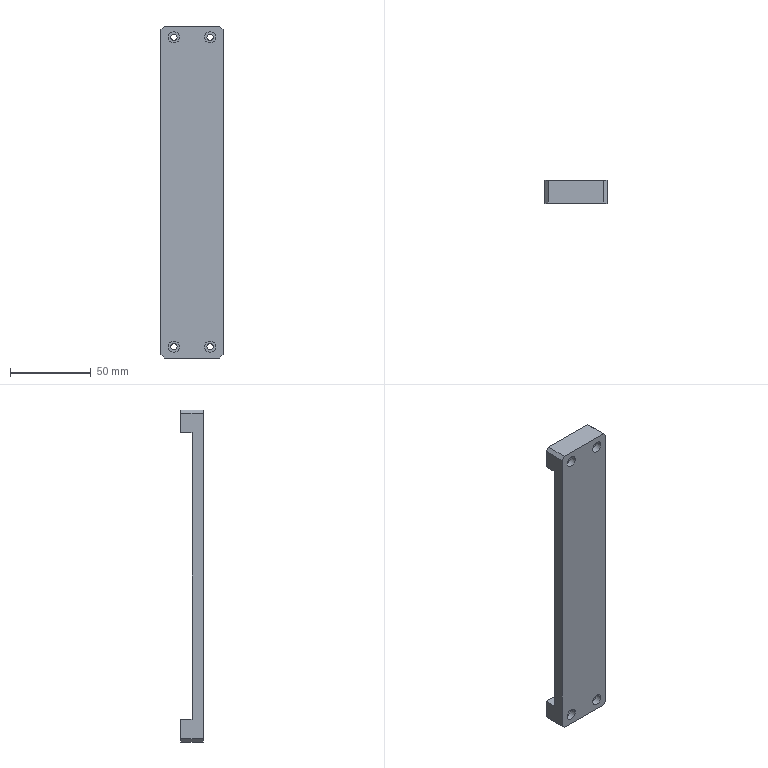Part | SolidWorks | features SplitBody 1 | 1 solid | 34 faces | box 38.5 x 14 x 205.8 mm | volume 61805 mm3 | plane 18 | cylinder 16 | commonest cylinder face diameters 3.85 x8 7 x8
STEP:
#1=CARTESIAN_POINT('',(1.625,218.849,-456.116));
#2=VERTEX_POINT('',#1);
#3=CARTESIAN_POINT('',(8.625,218.849,-456.116));
#4=VERTEX_POINT('',#3);
#5=CARTESIAN_POINT('',(5.125,218.849,-456.116));
#6=DIRECTION('',(0.,-1.,0.));
#7=DIRECTION('',(1.,0.,0.));
#8=AXIS2_PLACEMENT_3D('',#5,#6,#7);
#9=CIRCLE('',#8,3.5);
#10=EDGE_CURVE('',#2,#4,#9,.T.);
#11=ORIENTED_EDGE('',*,*,#10,.F.);
#12=CARTESIAN_POINT('',(1.625,214.859,-456.116));
#13=VERTEX_POINT('',#12);
#14=CARTESIAN_POINT('',(1.625,214.859,-456.116));
#15=DIRECTION('',(0.,-1.,0.));
#16=VECTOR('',#15,1000.);
#17=LINE('',#14,#16);
#18=EDGE_CURVE('',#2,#13,#17,.T.);
#19=ORIENTED_EDGE('',*,*,#18,.T.);
#20=CARTESIAN_POINT('',(8.625,214.859,-456.116));
#21=VERTEX_POINT('',#20);
#22=CARTESIAN_POINT('',(5.125,214.859,-456.116));
#23=DIRECTION('',(0.,-1.,0.));
#24=DIRECTION('',(1.,0.,0.));
#25=AXIS2_PLACEMENT_3D('',#22,#23,#24);
#26=CIRCLE('',#25,3.5);
#27=EDGE_CURVE('',#13,#21,#26,.T.);
#28=ORIENTED_EDGE('',*,*,#27,.T.);
#29=CARTESIAN_POINT('',(8.625,214.859,-456.116));
#30=DIRECTION('',(0.,-1.,0.));
#31=VECTOR('',#30,1000.);
#32=LINE('',#29,#31);
#33=EDGE_CURVE('',#4,#21,#32,.T.);
#34=ORIENTED_EDGE('',*,*,#33,.F.);
#35=EDGE_LOOP('',(#11,#19,#28,#34));
#36=FACE_OUTER_BOUND('',#35,.T.);
#37=CARTESIAN_POINT('',(5.125,214.859,-456.116));
#38=DIRECTION('',(0.,-1.,0.));
#39=DIRECTION('',(1.,0.,0.));
#40=AXIS2_PLACEMENT_3D('',#37,#38,#39);
#41=CYLINDRICAL_SURFACE('',#40,3.5);
#42=ADVANCED_FACE('',(#36),#41,.F.);
#43=CARTESIAN_POINT('',(3.2,228.859,-456.116));
#44=VERTEX_POINT('',#43);
#45=CARTESIAN_POINT('',(7.05,228.859,-456.116));
#46=VERTEX_POINT('',#45);
#47=CARTESIAN_POINT('',(5.125,228.859,-456.116));
#48=DIRECTION('',(0.,-1.,0.));
#49=DIRECTION('',(1.,0.,0.));
#50=AXIS2_PLACEMENT_3D('',#47,#48,#49);
#51=CIRCLE('',#50,1.925);
#52=EDGE_CURVE('',#44,#46,#51,.T.);
#53=ORIENTED_EDGE('',*,*,#52,.F.);
#54=CARTESIAN_POINT('',(3.2,218.849,-456.116));
#55=VERTEX_POINT('',#54);
#56=CARTESIAN_POINT('',(3.2,214.859,-456.116));
#57=DIRECTION('',(0.,-1.,0.));
#58=VECTOR('',#57,1000.);
#59=LINE('',#56,#58);
#60=EDGE_CURVE('',#44,#55,#59,.T.);
#61=ORIENTED_EDGE('',*,*,#60,.T.);
#62=CARTESIAN_POINT('',(7.05,218.849,-456.116));
#63=VERTEX_POINT('',#62);
#64=CARTESIAN_POINT('',(5.125,218.849,-456.116));
#65=DIRECTION('',(0.,-1.,0.));
#66=DIRECTION('',(1.,0.,0.));
#67=AXIS2_PLACEMENT_3D('',#64,#65,#66);
#68=CIRCLE('',#67,1.925);
#69=EDGE_CURVE('',#55,#63,#68,.T.);
#70=ORIENTED_EDGE('',*,*,#69,.T.);
#71=CARTESIAN_POINT('',(7.05,214.859,-456.116));
#72=DIRECTION('',(0.,-1.,0.));
#73=VECTOR('',#72,1000.);
#74=LINE('',#71,#73);
#75=EDGE_CURVE('',#46,#63,#74,.T.);
#76=ORIENTED_EDGE('',*,*,#75,.F.);
#77=EDGE_LOOP('',(#53,#61,#70,#76));
#78=FACE_OUTER_BOUND('',#77,.T.);
#79=CARTESIAN_POINT('',(5.125,214.859,-456.116));
#80=DIRECTION('',(0.,-1.,0.));
#81=DIRECTION('',(1.,0.,0.));
#82=AXIS2_PLACEMENT_3D('',#79,#80,#81);
#83=CYLINDRICAL_SURFACE('',#82,1.925);
#84=ADVANCED_FACE('',(#78),#83,.F.);
#85=CARTESIAN_POINT('',(24.025,218.849,-456.116));
#86=VERTEX_POINT('',#85);
#87=CARTESIAN_POINT('',(31.025,218.849,-456.116));
#88=VERTEX_POINT('',#87);
#89=CARTESIAN_POINT('',(27.525,218.849,-456.116));
#90=DIRECTION('',(0.,-1.,0.));
#91=DIRECTION('',(1.,0.,0.));
#92=AXIS2_PLACEMENT_3D('',#89,#90,#91);
#93=CIRCLE('',#92,3.5);
#94=EDGE_CURVE('',#86,#88,#93,.T.);
#95=ORIENTED_EDGE('',*,*,#94,.F.);
#96=CARTESIAN_POINT('',(24.025,214.859,-456.116));
#97=VERTEX_POINT('',#96);
#98=CARTESIAN_POINT('',(24.025,214.859,-456.116));
#99=DIRECTION('',(0.,-1.,0.));
#100=VECTOR('',#99,1000.);
#101=LINE('',#98,#100);
#102=EDGE_CURVE('',#86,#97,#101,.T.);
#103=ORIENTED_EDGE('',*,*,#102,.T.);
#104=CARTESIAN_POINT('',(31.025,214.859,-456.116));
#105=VERTEX_POINT('',#104);
#106=CARTESIAN_POINT('',(27.525,214.859,-456.116));
#107=DIRECTION('',(0.,-1.,0.));
#108=DIRECTION('',(1.,0.,0.));
#109=AXIS2_PLACEMENT_3D('',#106,#107,#108);
#110=CIRCLE('',#109,3.5);
#111=EDGE_CURVE('',#97,#105,#110,.T.);
#112=ORIENTED_EDGE('',*,*,#111,.T.);
#113=CARTESIAN_POINT('',(31.025,214.859,-456.116));
#114=DIRECTION('',(0.,-1.,0.));
#115=VECTOR('',#114,1000.);
#116=LINE('',#113,#115);
#117=EDGE_CURVE('',#88,#105,#116,.T.);
#118=ORIENTED_EDGE('',*,*,#117,.F.);
#119=EDGE_LOOP('',(#95,#103,#112,#118));
#120=FACE_OUTER_BOUND('',#119,.T.);
#121=CARTESIAN_POINT('',(27.525,214.859,-456.116));
#122=DIRECTION('',(0.,-1.,0.));
#123=DIRECTION('',(1.,0.,0.));
#124=AXIS2_PLACEMENT_3D('',#121,#122,#123);
#125=CYLINDRICAL_SURFACE('',#124,3.5);
#126=ADVANCED_FACE('',(#120),#125,.F.);
#127=CARTESIAN_POINT('',(25.6,228.859,-456.116));
#128=VERTEX_POINT('',#127);
#129=CARTESIAN_POINT('',(29.45,228.859,-456.116));
#130=VERTEX_POINT('',#129);
#131=CARTESIAN_POINT('',(27.525,228.859,-456.116));
#132=DIRECTION('',(0.,-1.,0.));
#133=DIRECTION('',(1.,0.,0.));
#134=AXIS2_PLACEMENT_3D('',#131,#132,#133);
#135=CIRCLE('',#134,1.925);
#136=EDGE_CURVE('',#128,#130,#135,.T.);
#137=ORIENTED_EDGE('',*,*,#136,.F.);
#138=CARTESIAN_POINT('',(25.6,218.849,-456.116));
#139=VERTEX_POINT('',#138);
#140=CARTESIAN_POINT('',(25.6,214.859,-456.116));
#141=DIRECTION('',(0.,-1.,0.));
#142=VECTOR('',#141,1000.);
#143=LINE('',#140,#142);
#144=EDGE_CURVE('',#128,#139,#143,.T.);
#145=ORIENTED_EDGE('',*,*,#144,.T.);
#146=CARTESIAN_POINT('',(29.45,218.849,-456.116));
#147=VERTEX_POINT('',#146);
#148=CARTESIAN_POINT('',(27.525,218.849,-456.116));
#149=DIRECTION('',(0.,-1.,0.));
#150=DIRECTION('',(1.,0.,0.));
#151=AXIS2_PLACEMENT_3D('',#148,#149,#150);
#152=CIRCLE('',#151,1.925);
#153=EDGE_CURVE('',#139,#147,#152,.T.);
#154=ORIENTED_EDGE('',*,*,#153,.T.);
#155=CARTESIAN_POINT('',(29.45,214.859,-456.116));
#156=DIRECTION('',(0.,-1.,0.));
#157=VECTOR('',#156,1000.);
#158=LINE('',#155,#157);
#159=EDGE_CURVE('',#130,#147,#158,.T.);
#160=ORIENTED_EDGE('',*,*,#159,.F.);
#161=EDGE_LOOP('',(#137,#145,#154,#160));
#162=FACE_OUTER_BOUND('',#161,.T.);
#163=CARTESIAN_POINT('',(27.525,214.859,-456.116));
#164=DIRECTION('',(0.,-1.,0.));
#165=DIRECTION('',(1.,0.,0.));
#166=AXIS2_PLACEMENT_3D('',#163,#164,#165);
#167=CYLINDRICAL_SURFACE('',#166,1.925);
#168=ADVANCED_FACE('',(#162),#167,.F.);
#169=CARTESIAN_POINT('',(1.625,218.849,-264.316));
#170=VERTEX_POINT('',#169);
#171=CARTESIAN_POINT('',(8.625,218.849,-264.316));
#172=VERTEX_POINT('',#171);
#173=CARTESIAN_POINT('',(5.125,218.849,-264.316));
#174=DIRECTION('',(0.,-1.,0.));
#175=DIRECTION('',(1.,0.,0.));
#176=AXIS2_PLACEMENT_3D('',#173,#174,#175);
#177=CIRCLE('',#176,3.5);
#178=EDGE_CURVE('',#170,#172,#177,.T.);
#179=ORIENTED_EDGE('',*,*,#178,.F.);
#180=CARTESIAN_POINT('',(1.625,214.859,-264.316));
#181=VERTEX_POINT('',#180);
#182=CARTESIAN_POINT('',(1.625,214.859,-264.316));
#183=DIRECTION('',(0.,-1.,0.));
#184=VECTOR('',#183,1000.);
#185=LINE('',#182,#184);
#186=EDGE_CURVE('',#170,#181,#185,.T.);
#187=ORIENTED_EDGE('',*,*,#186,.T.);
#188=CARTESIAN_POINT('',(8.625,214.859,-264.316));
#189=VERTEX_POINT('',#188);
#190=CARTESIAN_POINT('',(5.125,214.859,-264.316));
#191=DIRECTION('',(0.,-1.,0.));
#192=DIRECTION('',(1.,0.,0.));
#193=AXIS2_PLACEMENT_3D('',#190,#191,#192);
#194=CIRCLE('',#193,3.5);
#195=EDGE_CURVE('',#181,#189,#194,.T.);
#196=ORIENTED_EDGE('',*,*,#195,.T.);
#197=CARTESIAN_POINT('',(8.625,214.859,-264.316));
#198=DIRECTION('',(0.,-1.,0.));
#199=VECTOR('',#198,1000.);
#200=LINE('',#197,#199);
#201=EDGE_CURVE('',#172,#189,#200,.T.);
#202=ORIENTED_EDGE('',*,*,#201,.F.);
#203=EDGE_LOOP('',(#179,#187,#196,#202));
#204=FACE_OUTER_BOUND('',#203,.T.);
#205=CARTESIAN_POINT('',(5.125,214.859,-264.316));
#206=DIRECTION('',(0.,-1.,0.));
#207=DIRECTION('',(1.,0.,0.));
#208=AXIS2_PLACEMENT_3D('',#205,#206,#207);
#209=CYLINDRICAL_SURFACE('',#208,3.5);
#210=ADVANCED_FACE('',(#204),#209,.F.);
#211=CARTESIAN_POINT('',(3.2,228.859,-264.316));
#212=VERTEX_POINT('',#211);
#213=CARTESIAN_POINT('',(7.05,228.859,-264.316));
#214=VERTEX_POINT('',#213);
#215=CARTESIAN_POINT('',(5.125,228.859,-264.316));
#216=DIRECTION('',(0.,-1.,0.));
#217=DIRECTION('',(1.,0.,0.));
#218=AXIS2_PLACEMENT_3D('',#215,#216,#217);
#219=CIRCLE('',#218,1.925);
#220=EDGE_CURVE('',#212,#214,#219,.T.);
#221=ORIENTED_EDGE('',*,*,#220,.F.);
#222=CARTESIAN_POINT('',(3.2,218.849,-264.316));
#223=VERTEX_POINT('',#222);
#224=CARTESIAN_POINT('',(3.2,214.859,-264.316));
#225=DIRECTION('',(0.,-1.,0.));
#226=VECTOR('',#225,1000.);
#227=LINE('',#224,#226);
#228=EDGE_CURVE('',#212,#223,#227,.T.);
#229=ORIENTED_EDGE('',*,*,#228,.T.);
#230=CARTESIAN_POINT('',(7.05,218.849,-264.316));
#231=VERTEX_POINT('',#230);
#232=CARTESIAN_POINT('',(5.125,218.849,-264.316));
#233=DIRECTION('',(0.,-1.,0.));
#234=DIRECTION('',(1.,0.,0.));
#235=AXIS2_PLACEMENT_3D('',#232,#233,#234);
#236=CIRCLE('',#235,1.925);
#237=EDGE_CURVE('',#223,#231,#236,.T.);
#238=ORIENTED_EDGE('',*,*,#237,.T.);
#239=CARTESIAN_POINT('',(7.05,214.859,-264.316));
#240=DIRECTION('',(0.,-1.,0.));
#241=VECTOR('',#240,1000.);
#242=LINE('',#239,#241);
#243=EDGE_CURVE('',#214,#231,#242,.T.);
#244=ORIENTED_EDGE('',*,*,#243,.F.);
#245=EDGE_LOOP('',(#221,#229,#238,#244));
#246=FACE_OUTER_BOUND('',#245,.T.);
#247=CARTESIAN_POINT('',(5.125,214.859,-264.316));
#248=DIRECTION('',(0.,-1.,0.));
#249=DIRECTION('',(1.,0.,0.));
#250=AXIS2_PLACEMENT_3D('',#247,#248,#249);
#251=CYLINDRICAL_SURFACE('',#250,1.925);
#252=ADVANCED_FACE('',(#246),#251,.F.);
#253=CARTESIAN_POINT('',(24.025,218.849,-264.316));
#254=VERTEX_POINT('',#253);
#255=CARTESIAN_POINT('',(31.025,218.849,-264.316));
#256=VERTEX_POINT('',#255);
#257=CARTESIAN_POINT('',(27.525,218.849,-264.316));
#258=DIRECTION('',(0.,-1.,0.));
#259=DIRECTION('',(1.,0.,0.));
#260=AXIS2_PLACEMENT_3D('',#257,#258,#259);
#261=CIRCLE('',#260,3.5);
#262=EDGE_CURVE('',#254,#256,#261,.T.);
#263=ORIENTED_EDGE('',*,*,#262,.F.);
#264=CARTESIAN_POINT('',(24.025,214.859,-264.316));
#265=VERTEX_POINT('',#264);
#266=CARTESIAN_POINT('',(24.025,214.859,-264.316));
#267=DIRECTION('',(0.,-1.,0.));
#268=VECTOR('',#267,1000.);
#269=LINE('',#266,#268);
#270=EDGE_CURVE('',#254,#265,#269,.T.);
#271=ORIENTED_EDGE('',*,*,#270,.T.);
#272=CARTESIAN_POINT('',(31.025,214.859,-264.316));
#273=VERTEX_POINT('',#272);
#274=CARTESIAN_POINT('',(27.525,214.859,-264.316));
#275=DIRECTION('',(0.,-1.,0.));
#276=DIRECTION('',(1.,0.,0.));
#277=AXIS2_PLACEMENT_3D('',#274,#275,#276);
#278=CIRCLE('',#277,3.5);
#279=EDGE_CURVE('',#265,#273,#278,.T.);
#280=ORIENTED_EDGE('',*,*,#279,.T.);
#281=CARTESIAN_POINT('',(31.025,214.859,-264.316));
#282=DIRECTION('',(0.,-1.,0.));
#283=VECTOR('',#282,1000.);
#284=LINE('',#281,#283);
#285=EDGE_CURVE('',#256,#273,#284,.T.);
#286=ORIENTED_EDGE('',*,*,#285,.F.);
#287=EDGE_LOOP('',(#263,#271,#280,#286));
#288=FACE_OUTER_BOUND('',#287,.T.);
#289=CARTESIAN_POINT('',(27.525,214.859,-264.316));
#290=DIRECTION('',(0.,-1.,0.));
#291=DIRECTION('',(1.,0.,0.));
#292=AXIS2_PLACEMENT_3D('',#289,#290,#291);
#293=CYLINDRICAL_SURFACE('',#292,3.5);
#294=ADVANCED_FACE('',(#288),#293,.F.);
#295=CARTESIAN_POINT('',(25.6,228.859,-264.316));
#296=VERTEX_POINT('',#295);
#297=CARTESIAN_POINT('',(29.45,228.859,-264.316));
#298=VERTEX_POINT('',#297);
#299=CARTESIAN_POINT('',(27.525,228.859,-264.316));
#300=DIRECTION('',(0.,-1.,0.));
#301=DIRECTION('',(1.,0.,0.));
#302=AXIS2_PLACEMENT_3D('',#299,#300,#301);
#303=CIRCLE('',#302,1.925);
#304=EDGE_CURVE('',#296,#298,#303,.T.);
#305=ORIENTED_EDGE('',*,*,#304,.F.);
#306=CARTESIAN_POINT('',(25.6,218.849,-264.316));
#307=VERTEX_POINT('',#306);
#308=CARTESIAN_POINT('',(25.6,214.859,-264.316));
#309=DIRECTION('',(0.,-1.,0.));
#310=VECTOR('',#309,1000.);
#311=LINE('',#308,#310);
#312=EDGE_CURVE('',#296,#307,#311,.T.);
#313=ORIENTED_EDGE('',*,*,#312,.T.);
#314=CARTESIAN_POINT('',(29.45,218.849,-264.316));
#315=VERTEX_POINT('',#314);
#316=CARTESIAN_POINT('',(27.525,218.849,-264.316));
#317=DIRECTION('',(0.,-1.,0.));
#318=DIRECTION('',(1.,0.,0.));
#319=AXIS2_PLACEMENT_3D('',#316,#317,#318);
#320=CIRCLE('',#319,1.925);
#321=EDGE_CURVE('',#307,#315,#320,.T.);
#322=ORIENTED_EDGE('',*,*,#321,.T.);
#323=CARTESIAN_POINT('',(29.45,214.859,-264.316));
#324=DIRECTION('',(0.,-1.,0.));
#325=VECTOR('',#324,1000.);
#326=LINE('',#323,#325);
#327=EDGE_CURVE('',#298,#315,#326,.T.);
#328=ORIENTED_EDGE('',*,*,#327,.F.);
#329=EDGE_LOOP('',(#305,#313,#322,#328));
#330=FACE_OUTER_BOUND('',#329,.T.);
#331=CARTESIAN_POINT('',(27.525,214.859,-264.316));
#332=DIRECTION('',(0.,-1.,0.));
#333=DIRECTION('',(1.,0.,0.));
#334=AXIS2_PLACEMENT_3D('',#331,#332,#333);
#335=CYLINDRICAL_SURFACE('',#334,1.925);
#336=ADVANCED_FACE('',(#330),#335,.F.);
#337=CARTESIAN_POINT('',(-0.8247,228.859,-463.116));
#338=VERTEX_POINT('',#337);
#339=CARTESIAN_POINT('',(33.475,228.859,-463.116));
#340=VERTEX_POINT('',#339);
#341=CARTESIAN_POINT('',(-2.925,228.859,-463.116));
#342=DIRECTION('',(1.,0.,0.));
#343=VECTOR('',#342,1000.);
#344=LINE('',#341,#343);
#345=EDGE_CURVE('',#338,#340,#344,.T.);
#346=ORIENTED_EDGE('',*,*,#345,.T.);
#347=CARTESIAN_POINT('',(33.475,214.859,-463.116));
#348=VERTEX_POINT('',#347);
#349=CARTESIAN_POINT('',(33.475,214.859,-463.116));
#350=DIRECTION('',(0.,-1.,0.));
#351=VECTOR('',#350,1000.);
#352=LINE('',#349,#351);
#353=EDGE_CURVE('',#340,#348,#352,.T.);
#354=ORIENTED_EDGE('',*,*,#353,.T.);
#355=CARTESIAN_POINT('',(-0.8247,214.859,-463.116));
#356=VERTEX_POINT('',#355);
#357=CARTESIAN_POINT('',(-2.925,214.859,-463.116));
#358=DIRECTION('',(1.,0.,0.));
#359=VECTOR('',#358,1000.);
#360=LINE('',#357,#359);
#361=EDGE_CURVE('',#356,#348,#360,.T.);
#362=ORIENTED_EDGE('',*,*,#361,.F.);
#363=CARTESIAN_POINT('',(-0.8247,214.859,-463.116));
#364=DIRECTION('',(0.,1.,0.));
#365=VECTOR('',#364,1000.);
#366=LINE('',#363,#365);
#367=EDGE_CURVE('',#356,#338,#366,.T.);
#368=ORIENTED_EDGE('',*,*,#367,.T.);
#369=EDGE_LOOP('',(#346,#354,#362,#368));
#370=FACE_OUTER_BOUND('',#369,.T.);
#371=CARTESIAN_POINT('',(-2.925,214.859,-463.116));
#372=DIRECTION('',(0.,0.,1.));
#373=DIRECTION('',(1.,0.,0.));
#374=AXIS2_PLACEMENT_3D('',#371,#372,#373);
#375=PLANE('',#374);
#376=ADVANCED_FACE('',(#370),#375,.F.);
#377=CARTESIAN_POINT('',(5.125,214.859,-456.116));
#378=DIRECTION('',(0.,-1.,0.));
#379=DIRECTION('',(1.,0.,0.));
#380=AXIS2_PLACEMENT_3D('',#377,#378,#379);
#381=CIRCLE('',#380,3.5);
#382=EDGE_CURVE('',#21,#13,#381,.T.);
#383=ORIENTED_EDGE('',*,*,#382,.F.);
#384=ORIENTED_EDGE('',*,*,#27,.F.);
#385=EDGE_LOOP('',(#383,#384));
#386=FACE_BOUND('',#385,.T.);
#387=CARTESIAN_POINT('',(27.525,214.859,-456.116));
#388=DIRECTION('',(0.,-1.,0.));
#389=DIRECTION('',(1.,0.,0.));
#390=AXIS2_PLACEMENT_3D('',#387,#388,#389);
#391=CIRCLE('',#390,3.5);
#392=EDGE_CURVE('',#105,#97,#391,.T.);
#393=ORIENTED_EDGE('',*,*,#392,.F.);
#394=ORIENTED_EDGE('',*,*,#111,.F.);
#395=EDGE_LOOP('',(#393,#394));
#396=FACE_BOUND('',#395,.T.);
#397=CARTESIAN_POINT('',(5.125,214.859,-264.316));
#398=DIRECTION('',(0.,-1.,0.));
#399=DIRECTION('',(1.,0.,0.));
#400=AXIS2_PLACEMENT_3D('',#397,#398,#399);
#401=CIRCLE('',#400,3.5);
#402=EDGE_CURVE('',#189,#181,#401,.T.);
#403=ORIENTED_EDGE('',*,*,#402,.F.);
#404=ORIENTED_EDGE('',*,*,#195,.F.);
#405=EDGE_LOOP('',(#403,#404));
#406=FACE_BOUND('',#405,.T.);
#407=CARTESIAN_POINT('',(27.525,214.859,-264.316));
#408=DIRECTION('',(0.,-1.,0.));
#409=DIRECTION('',(1.,0.,0.));
#410=AXIS2_PLACEMENT_3D('',#407,#408,#409);
#411=CIRCLE('',#410,3.5);
#412=EDGE_CURVE('',#273,#265,#411,.T.);
#413=ORIENTED_EDGE('',*,*,#412,.F.);
#414=ORIENTED_EDGE('',*,*,#279,.F.);
#415=EDGE_LOOP('',(#413,#414));
#416=FACE_BOUND('',#415,.T.);
#417=CARTESIAN_POINT('',(35.575,214.859,-461.016));
#418=VERTEX_POINT('',#417);
#419=CARTESIAN_POINT('',(35.575,214.859,-259.416));
#420=VERTEX_POINT('',#419);
#421=CARTESIAN_POINT('',(35.575,214.859,-463.116));
#422=DIRECTION('',(0.,0.,1.));
#423=VECTOR('',#422,1000.);
#424=LINE('',#421,#423);
#425=EDGE_CURVE('',#418,#420,#424,.T.);
#426=ORIENTED_EDGE('',*,*,#425,.T.);
#427=CARTESIAN_POINT('',(33.475,214.859,-257.316));
#428=VERTEX_POINT('',#427);
#429=CARTESIAN_POINT('',(33.475,214.859,-257.316));
#430=DIRECTION('',(-0.7071,0.,0.7071));
#431=VECTOR('',#430,1000.);
#432=LINE('',#429,#431);
#433=EDGE_CURVE('',#420,#428,#432,.T.);
#434=ORIENTED_EDGE('',*,*,#433,.T.);
#435=CARTESIAN_POINT('',(-0.8247,214.859,-257.316));
#436=VERTEX_POINT('',#435);
#437=CARTESIAN_POINT('',(-2.925,214.859,-257.316));
#438=DIRECTION('',(1.,0.,0.));
#439=VECTOR('',#438,1000.);
#440=LINE('',#437,#439);
#441=EDGE_CURVE('',#436,#428,#440,.T.);
#442=ORIENTED_EDGE('',*,*,#441,.F.);
#443=CARTESIAN_POINT('',(-2.925,214.859,-259.416));
#444=VERTEX_POINT('',#443);
#445=CARTESIAN_POINT('',(-2.925,214.859,-259.416));
#446=DIRECTION('',(-0.7071,0.,-0.7071));
#447=VECTOR('',#446,1000.);
#448=LINE('',#445,#447);
#449=EDGE_CURVE('',#436,#444,#448,.T.);
#450=ORIENTED_EDGE('',*,*,#449,.T.);
#451=CARTESIAN_POINT('',(-2.925,214.859,-461.016));
#452=VERTEX_POINT('',#451);
#453=CARTESIAN_POINT('',(-2.925,214.859,-463.116));
#454=DIRECTION('',(0.,0.,1.));
#455=VECTOR('',#454,1000.);
#456=LINE('',#453,#455);
#457=EDGE_CURVE('',#452,#444,#456,.T.);
#458=ORIENTED_EDGE('',*,*,#457,.F.);
#459=CARTESIAN_POINT('',(-2.925,214.859,-461.016));
#460=DIRECTION('',(0.7071,0.,-0.7071));
#461=VECTOR('',#460,1000.);
#462=LINE('',#459,#461);
#463=EDGE_CURVE('',#452,#356,#462,.T.);
#464=ORIENTED_EDGE('',*,*,#463,.T.);
#465=ORIENTED_EDGE('',*,*,#361,.T.);
#466=CARTESIAN_POINT('',(33.475,214.859,-463.116));
#467=DIRECTION('',(0.7071,0.,0.7071));
#468=VECTOR('',#467,1000.);
#469=LINE('',#466,#468);
#470=EDGE_CURVE('',#348,#418,#469,.T.);
#471=ORIENTED_EDGE('',*,*,#470,.T.);
#472=EDGE_LOOP('',(#426,#434,#442,#450,#458,#464,#465,#471));
#473=FACE_OUTER_BOUND('',#472,.T.);
#474=CARTESIAN_POINT('',(-2.925,214.859,-463.116));
#475=DIRECTION('',(0.,1.,0.));
#476=DIRECTION('',(-1.,0.,0.));
#477=AXIS2_PLACEMENT_3D('',#474,#475,#476);
#478=PLANE('',#477);
#479=ADVANCED_FACE('',(#386,#396,#406,#416,#473),#478,.F.);
#480=ORIENTED_EDGE('',*,*,#441,.T.);
#481=CARTESIAN_POINT('',(33.475,228.859,-257.316));
#482=VERTEX_POINT('',#481);
#483=CARTESIAN_POINT('',(33.475,228.859,-257.316));
#484=DIRECTION('',(0.,1.,0.));
#485=VECTOR('',#484,1000.);
#486=LINE('',#483,#485);
#487=EDGE_CURVE('',#428,#482,#486,.T.);
#488=ORIENTED_EDGE('',*,*,#487,.T.);
#489=CARTESIAN_POINT('',(-0.8247,228.859,-257.316));
#490=VERTEX_POINT('',#489);
#491=CARTESIAN_POINT('',(-2.925,228.859,-257.316));
#492=DIRECTION('',(1.,0.,0.));
#493=VECTOR('',#492,1000.);
#494=LINE('',#491,#493);
#495=EDGE_CURVE('',#490,#482,#494,.T.);
#496=ORIENTED_EDGE('',*,*,#495,.F.);
#497=CARTESIAN_POINT('',(-0.8247,214.859,-257.316));
#498=DIRECTION('',(0.,-1.,0.));
#499=VECTOR('',#498,1000.);
#500=LINE('',#497,#499);
#501=EDGE_CURVE('',#490,#436,#500,.T.);
#502=ORIENTED_EDGE('',*,*,#501,.T.);
#503=EDGE_LOOP('',(#480,#488,#496,#502));
#504=FACE_OUTER_BOUND('',#503,.T.);
#505=CARTESIAN_POINT('',(-2.925,214.859,-257.316));
#506=DIRECTION('',(0.,0.,-1.));
#507=DIRECTION('',(-1.,0.,0.));
#508=AXIS2_PLACEMENT_3D('',#505,#506,#507);
#509=PLANE('',#508);
#510=ADVANCED_FACE('',(#504),#509,.F.);
#511=CARTESIAN_POINT('',(5.125,228.859,-264.316));
#512=DIRECTION('',(0.,-1.,0.));
#513=DIRECTION('',(1.,0.,0.));
#514=AXIS2_PLACEMENT_3D('',#511,#512,#513);
#515=CIRCLE('',#514,1.925);
#516=EDGE_CURVE('',#214,#212,#515,.T.);
#517=ORIENTED_EDGE('',*,*,#516,.T.);
#518=ORIENTED_EDGE('',*,*,#220,.T.);
#519=EDGE_LOOP('',(#517,#518));
#520=FACE_BOUND('',#519,.T.);
#521=CARTESIAN_POINT('',(27.525,228.859,-264.316));
#522=DIRECTION('',(0.,-1.,0.));
#523=DIRECTION('',(1.,0.,0.));
#524=AXIS2_PLACEMENT_3D('',#521,#522,#523);
#525=CIRCLE('',#524,1.925);
#526=EDGE_CURVE('',#298,#296,#525,.T.);
#527=ORIENTED_EDGE('',*,*,#526,.T.);
#528=ORIENTED_EDGE('',*,*,#304,.T.);
#529=EDGE_LOOP('',(#527,#528));
#530=FACE_BOUND('',#529,.T.);
#531=ORIENTED_EDGE('',*,*,#495,.T.);
#532=CARTESIAN_POINT('',(35.575,228.859,-259.416));
#533=VERTEX_POINT('',#532);
#534=CARTESIAN_POINT('',(33.475,228.859,-257.316));
#535=DIRECTION('',(0.7071,0.,-0.7071));
#536=VECTOR('',#535,1000.);
#537=LINE('',#534,#536);
#538=EDGE_CURVE('',#482,#533,#537,.T.);
#539=ORIENTED_EDGE('',*,*,#538,.T.);
#540=CARTESIAN_POINT('',(35.575,228.859,-271.316));
#541=VERTEX_POINT('',#540);
#542=CARTESIAN_POINT('',(35.575,228.859,-271.316));
#543=DIRECTION('',(0.,0.,-1.));
#544=VECTOR('',#543,1000.);
#545=LINE('',#542,#544);
#546=EDGE_CURVE('',#533,#541,#545,.T.);
#547=ORIENTED_EDGE('',*,*,#546,.T.);
#548=CARTESIAN_POINT('',(-2.925,228.859,-271.316));
#549=VERTEX_POINT('',#548);
#550=CARTESIAN_POINT('',(-2.925,228.859,-271.316));
#551=DIRECTION('',(1.,0.,0.));
#552=VECTOR('',#551,1000.);
#553=LINE('',#550,#552);
#554=EDGE_CURVE('',#549,#541,#553,.T.);
#555=ORIENTED_EDGE('',*,*,#554,.F.);
#556=CARTESIAN_POINT('',(-2.925,228.859,-259.416));
#557=VERTEX_POINT('',#556);
#558=CARTESIAN_POINT('',(-2.925,228.859,-271.316));
#559=DIRECTION('',(0.,0.,-1.));
#560=VECTOR('',#559,1000.);
#561=LINE('',#558,#560);
#562=EDGE_CURVE('',#557,#549,#561,.T.);
#563=ORIENTED_EDGE('',*,*,#562,.F.);
#564=CARTESIAN_POINT('',(-2.925,228.859,-259.416));
#565=DIRECTION('',(0.7071,0.,0.7071));
#566=VECTOR('',#565,1000.);
#567=LINE('',#564,#566);
#568=EDGE_CURVE('',#557,#490,#567,.T.);
#569=ORIENTED_EDGE('',*,*,#568,.T.);
#570=EDGE_LOOP('',(#531,#539,#547,#555,#563,#569));
#571=FACE_OUTER_BOUND('',#570,.T.);
#572=CARTESIAN_POINT('',(-2.925,228.859,-271.316));
#573=DIRECTION('',(0.,-1.,0.));
#574=DIRECTION('',(1.,0.,0.));
#575=AXIS2_PLACEMENT_3D('',#572,#573,#574);
#576=PLANE('',#575);
#577=ADVANCED_FACE('',(#520,#530,#571),#576,.F.);
#578=CARTESIAN_POINT('',(35.575,221.859,-271.316));
#579=VERTEX_POINT('',#578);
#580=CARTESIAN_POINT('',(35.575,228.859,-271.316));
#581=DIRECTION('',(0.,-1.,0.));
#582=VECTOR('',#581,1000.);
#583=LINE('',#580,#582);
#584=EDGE_CURVE('',#541,#579,#583,.T.);
#585=ORIENTED_EDGE('',*,*,#584,.T.);
#586=CARTESIAN_POINT('',(-2.925,221.859,-271.316));
#587=VERTEX_POINT('',#586);
#588=CARTESIAN_POINT('',(-2.925,221.859,-271.316));
#589=DIRECTION('',(1.,0.,0.));
#590=VECTOR('',#589,1000.);
#591=LINE('',#588,#590);
#592=EDGE_CURVE('',#587,#579,#591,.T.);
#593=ORIENTED_EDGE('',*,*,#592,.F.);
#594=CARTESIAN_POINT('',(-2.925,228.859,-271.316));
#595=DIRECTION('',(0.,-1.,0.));
#596=VECTOR('',#595,1000.);
#597=LINE('',#594,#596);
#598=EDGE_CURVE('',#549,#587,#597,.T.);
#599=ORIENTED_EDGE('',*,*,#598,.F.);
#600=ORIENTED_EDGE('',*,*,#554,.T.);
#601=EDGE_LOOP('',(#585,#593,#599,#600));
#602=FACE_OUTER_BOUND('',#601,.T.);
#603=CARTESIAN_POINT('',(-2.925,228.859,-271.316));
#604=DIRECTION('',(0.,0.,1.));
#605=DIRECTION('',(1.,0.,0.));
#606=AXIS2_PLACEMENT_3D('',#603,#604,#605);
#607=PLANE('',#606);
#608=ADVANCED_FACE('',(#602),#607,.F.);
#609=CARTESIAN_POINT('',(35.575,221.859,-449.116));
#610=VERTEX_POINT('',#609);
#611=CARTESIAN_POINT('',(35.575,221.859,-449.116));
#612=DIRECTION('',(0.,0.,-1.));
#613=VECTOR('',#612,1000.);
#614=LINE('',#611,#613);
#615=EDGE_CURVE('',#579,#610,#614,.T.);
#616=ORIENTED_EDGE('',*,*,#615,.T.);
#617=CARTESIAN_POINT('',(-2.925,221.859,-449.116));
#618=VERTEX_POINT('',#617);
#619=CARTESIAN_POINT('',(-2.925,221.859,-449.116));
#620=DIRECTION('',(1.,0.,0.));
#621=VECTOR('',#620,1000.);
#622=LINE('',#619,#621);
#623=EDGE_CURVE('',#618,#610,#622,.T.);
#624=ORIENTED_EDGE('',*,*,#623,.F.);
#625=CARTESIAN_POINT('',(-2.925,221.859,-449.116));
#626=DIRECTION('',(0.,0.,-1.));
#627=VECTOR('',#626,1000.);
#628=LINE('',#625,#627);
#629=EDGE_CURVE('',#587,#618,#628,.T.);
#630=ORIENTED_EDGE('',*,*,#629,.F.);
#631=ORIENTED_EDGE('',*,*,#592,.T.);
#632=EDGE_LOOP('',(#616,#624,#630,#631));
#633=FACE_OUTER_BOUND('',#632,.T.);
#634=CARTESIAN_POINT('',(-2.925,221.859,-449.116));
#635=DIRECTION('',(0.,-1.,0.));
#636=DIRECTION('',(1.,0.,0.));
#637=AXIS2_PLACEMENT_3D('',#634,#635,#636);
#638=PLANE('',#637);
#639=ADVANCED_FACE('',(#633),#638,.F.);
#640=CARTESIAN_POINT('',(35.575,228.859,-449.116));
#641=VERTEX_POINT('',#640);
#642=CARTESIAN_POINT('',(35.575,228.859,-449.116));
#643=DIRECTION('',(0.,1.,0.));
#644=VECTOR('',#643,1000.);
#645=LINE('',#642,#644);
#646=EDGE_CURVE('',#610,#641,#645,.T.);
#647=ORIENTED_EDGE('',*,*,#646,.T.);
#648=CARTESIAN_POINT('',(-2.925,228.859,-449.116));
#649=VERTEX_POINT('',#648);
#650=CARTESIAN_POINT('',(-2.925,228.859,-449.116));
#651=DIRECTION('',(1.,0.,0.));
#652=VECTOR('',#651,1000.);
#653=LINE('',#650,#652);
#654=EDGE_CURVE('',#649,#641,#653,.T.);
#655=ORIENTED_EDGE('',*,*,#654,.F.);
#656=CARTESIAN_POINT('',(-2.925,228.859,-449.116));
#657=DIRECTION('',(0.,1.,0.));
#658=VECTOR('',#657,1000.);
#659=LINE('',#656,#658);
#660=EDGE_CURVE('',#618,#649,#659,.T.);
#661=ORIENTED_EDGE('',*,*,#660,.F.);
#662=ORIENTED_EDGE('',*,*,#623,.T.);
#663=EDGE_LOOP('',(#647,#655,#661,#662));
#664=FACE_OUTER_BOUND('',#663,.T.);
#665=CARTESIAN_POINT('',(-2.925,228.859,-449.116));
#666=DIRECTION('',(0.,0.,-1.));
#667=DIRECTION('',(-1.,0.,0.));
#668=AXIS2_PLACEMENT_3D('',#665,#666,#667);
#669=PLANE('',#668);
#670=ADVANCED_FACE('',(#664),#669,.F.);
#671=CARTESIAN_POINT('',(5.125,228.859,-456.116));
#672=DIRECTION('',(0.,-1.,0.));
#673=DIRECTION('',(1.,0.,0.));
#674=AXIS2_PLACEMENT_3D('',#671,#672,#673);
#675=CIRCLE('',#674,1.925);
#676=EDGE_CURVE('',#46,#44,#675,.T.);
#677=ORIENTED_EDGE('',*,*,#676,.T.);
#678=ORIENTED_EDGE('',*,*,#52,.T.);
#679=EDGE_LOOP('',(#677,#678));
#680=FACE_BOUND('',#679,.T.);
#681=CARTESIAN_POINT('',(27.525,228.859,-456.116));
#682=DIRECTION('',(0.,-1.,0.));
#683=DIRECTION('',(1.,0.,0.));
#684=AXIS2_PLACEMENT_3D('',#681,#682,#683);
#685=CIRCLE('',#684,1.925);
#686=EDGE_CURVE('',#130,#128,#685,.T.);
#687=ORIENTED_EDGE('',*,*,#686,.T.);
#688=ORIENTED_EDGE('',*,*,#136,.T.);
#689=EDGE_LOOP('',(#687,#688));
#690=FACE_BOUND('',#689,.T.);
#691=CARTESIAN_POINT('',(35.575,228.859,-461.016));
#692=VERTEX_POINT('',#691);
#693=CARTESIAN_POINT('',(35.575,228.859,-463.116));
#694=DIRECTION('',(0.,0.,-1.));
#695=VECTOR('',#694,1000.);
#696=LINE('',#693,#695);
#697=EDGE_CURVE('',#641,#692,#696,.T.);
#698=ORIENTED_EDGE('',*,*,#697,.T.);
#699=CARTESIAN_POINT('',(33.475,228.859,-463.116));
#700=DIRECTION('',(-0.7071,0.,-0.7071));
#701=VECTOR('',#700,1000.);
#702=LINE('',#699,#701);
#703=EDGE_CURVE('',#692,#340,#702,.T.);
#704=ORIENTED_EDGE('',*,*,#703,.T.);
#705=ORIENTED_EDGE('',*,*,#345,.F.);
#706=CARTESIAN_POINT('',(-2.925,228.859,-461.016));
#707=VERTEX_POINT('',#706);
#708=CARTESIAN_POINT('',(-2.925,228.859,-461.016));
#709=DIRECTION('',(-0.7071,0.,0.7071));
#710=VECTOR('',#709,1000.);
#711=LINE('',#708,#710);
#712=EDGE_CURVE('',#338,#707,#711,.T.);
#713=ORIENTED_EDGE('',*,*,#712,.T.);
#714=CARTESIAN_POINT('',(-2.925,228.859,-463.116));
#715=DIRECTION('',(0.,0.,-1.));
#716=VECTOR('',#715,1000.);
#717=LINE('',#714,#716);
#718=EDGE_CURVE('',#649,#707,#717,.T.);
#719=ORIENTED_EDGE('',*,*,#718,.F.);
#720=ORIENTED_EDGE('',*,*,#654,.T.);
#721=EDGE_LOOP('',(#698,#704,#705,#713,#719,#720));
#722=FACE_OUTER_BOUND('',#721,.T.);
#723=CARTESIAN_POINT('',(-2.925,228.859,-463.116));
#724=DIRECTION('',(0.,-1.,0.));
#725=DIRECTION('',(1.,0.,0.));
#726=AXIS2_PLACEMENT_3D('',#723,#724,#725);
#727=PLANE('',#726);
#728=ADVANCED_FACE('',(#680,#690,#722),#727,.F.);
#729=ORIENTED_EDGE('',*,*,#457,.T.);
#730=CARTESIAN_POINT('',(-2.925,228.859,-259.416));
#731=DIRECTION('',(0.,1.,0.));
#732=VECTOR('',#731,1000.);
#733=LINE('',#730,#732);
#734=EDGE_CURVE('',#444,#557,#733,.T.);
#735=ORIENTED_EDGE('',*,*,#734,.T.);
#736=ORIENTED_EDGE('',*,*,#562,.T.);
#737=ORIENTED_EDGE('',*,*,#598,.T.);
#738=ORIENTED_EDGE('',*,*,#629,.T.);
#739=ORIENTED_EDGE('',*,*,#660,.T.);
#740=ORIENTED_EDGE('',*,*,#718,.T.);
#741=CARTESIAN_POINT('',(-2.925,228.859,-461.016));
#742=DIRECTION('',(0.,-1.,0.));
#743=VECTOR('',#742,1000.);
#744=LINE('',#741,#743);
#745=EDGE_CURVE('',#707,#452,#744,.T.);
#746=ORIENTED_EDGE('',*,*,#745,.T.);
#747=EDGE_LOOP('',(#729,#735,#736,#737,#738,#739,#740,#746));
#748=FACE_OUTER_BOUND('',#747,.T.);
#749=CARTESIAN_POINT('',(-2.925,228.859,-463.116));
#750=DIRECTION('',(1.,0.,0.));
#751=DIRECTION('',(0.,0.,-1.));
#752=AXIS2_PLACEMENT_3D('',#749,#750,#751);
#753=PLANE('',#752);
#754=ADVANCED_FACE('',(#748),#753,.F.);
#755=ORIENTED_EDGE('',*,*,#546,.F.);
#756=CARTESIAN_POINT('',(35.575,214.859,-259.416));
#757=DIRECTION('',(0.,-1.,0.));
#758=VECTOR('',#757,1000.);
#759=LINE('',#756,#758);
#760=EDGE_CURVE('',#533,#420,#759,.T.);
#761=ORIENTED_EDGE('',*,*,#760,.T.);
#762=ORIENTED_EDGE('',*,*,#425,.F.);
#763=CARTESIAN_POINT('',(35.575,228.859,-461.016));
#764=DIRECTION('',(0.,1.,0.));
#765=VECTOR('',#764,1000.);
#766=LINE('',#763,#765);
#767=EDGE_CURVE('',#418,#692,#766,.T.);
#768=ORIENTED_EDGE('',*,*,#767,.T.);
#769=ORIENTED_EDGE('',*,*,#697,.F.);
#770=ORIENTED_EDGE('',*,*,#646,.F.);
#771=ORIENTED_EDGE('',*,*,#615,.F.);
#772=ORIENTED_EDGE('',*,*,#584,.F.);
#773=EDGE_LOOP('',(#755,#761,#762,#768,#769,#770,#771,#772));
#774=FACE_OUTER_BOUND('',#773,.T.);
#775=CARTESIAN_POINT('',(35.575,228.859,-463.116));
#776=DIRECTION('',(1.,0.,0.));
#777=DIRECTION('',(0.,0.,-1.));
#778=AXIS2_PLACEMENT_3D('',#775,#776,#777);
#779=PLANE('',#778);
#780=ADVANCED_FACE('',(#774),#779,.T.);
#781=ORIENTED_EDGE('',*,*,#312,.F.);
#782=ORIENTED_EDGE('',*,*,#526,.F.);
#783=ORIENTED_EDGE('',*,*,#327,.T.);
#784=CARTESIAN_POINT('',(27.525,218.849,-264.316));
#785=DIRECTION('',(0.,-1.,0.));
#786=DIRECTION('',(1.,0.,0.));
#787=AXIS2_PLACEMENT_3D('',#784,#785,#786);
#788=CIRCLE('',#787,1.925);
#789=EDGE_CURVE('',#315,#307,#788,.T.);
#790=ORIENTED_EDGE('',*,*,#789,.T.);
#791=EDGE_LOOP('',(#781,#782,#783,#790));
#792=FACE_OUTER_BOUND('',#791,.T.);
#793=CARTESIAN_POINT('',(27.525,214.859,-264.316));
#794=DIRECTION('',(0.,-1.,0.));
#795=DIRECTION('',(1.,0.,0.));
#796=AXIS2_PLACEMENT_3D('',#793,#794,#795);
#797=CYLINDRICAL_SURFACE('',#796,1.925);
#798=ADVANCED_FACE('',(#792),#797,.F.);
#799=ORIENTED_EDGE('',*,*,#789,.F.);
#800=ORIENTED_EDGE('',*,*,#321,.F.);
#801=EDGE_LOOP('',(#799,#800));
#802=FACE_BOUND('',#801,.T.);
#803=CARTESIAN_POINT('',(27.525,218.849,-264.316));
#804=DIRECTION('',(0.,-1.,0.));
#805=DIRECTION('',(1.,0.,0.));
#806=AXIS2_PLACEMENT_3D('',#803,#804,#805);
#807=CIRCLE('',#806,3.5);
#808=EDGE_CURVE('',#256,#254,#807,.T.);
#809=ORIENTED_EDGE('',*,*,#808,.T.);
#810=ORIENTED_EDGE('',*,*,#262,.T.);
#811=EDGE_LOOP('',(#809,#810));
#812=FACE_OUTER_BOUND('',#811,.T.);
#813=CARTESIAN_POINT('',(27.525,218.849,-262.391));
#814=DIRECTION('',(0.,1.,0.));
#815=DIRECTION('',(-1.,0.,0.));
#816=AXIS2_PLACEMENT_3D('',#813,#814,#815);
#817=PLANE('',#816);
#818=ADVANCED_FACE('',(#802,#812),#817,.F.);
#819=ORIENTED_EDGE('',*,*,#270,.F.);
#820=ORIENTED_EDGE('',*,*,#808,.F.);
#821=ORIENTED_EDGE('',*,*,#285,.T.);
#822=ORIENTED_EDGE('',*,*,#412,.T.);
#823=EDGE_LOOP('',(#819,#820,#821,#822));
#824=FACE_OUTER_BOUND('',#823,.T.);
#825=CARTESIAN_POINT('',(27.525,214.859,-264.316));
#826=DIRECTION('',(0.,-1.,0.));
#827=DIRECTION('',(1.,0.,0.));
#828=AXIS2_PLACEMENT_3D('',#825,#826,#827);
#829=CYLINDRICAL_SURFACE('',#828,3.5);
#830=ADVANCED_FACE('',(#824),#829,.F.);
#831=ORIENTED_EDGE('',*,*,#228,.F.);
#832=ORIENTED_EDGE('',*,*,#516,.F.);
#833=ORIENTED_EDGE('',*,*,#243,.T.);
#834=CARTESIAN_POINT('',(5.125,218.849,-264.316));
#835=DIRECTION('',(0.,-1.,0.));
#836=DIRECTION('',(1.,0.,0.));
#837=AXIS2_PLACEMENT_3D('',#834,#835,#836);
#838=CIRCLE('',#837,1.925);
#839=EDGE_CURVE('',#231,#223,#838,.T.);
#840=ORIENTED_EDGE('',*,*,#839,.T.);
#841=EDGE_LOOP('',(#831,#832,#833,#840));
#842=FACE_OUTER_BOUND('',#841,.T.);
#843=CARTESIAN_POINT('',(5.125,214.859,-264.316));
#844=DIRECTION('',(0.,-1.,0.));
#845=DIRECTION('',(1.,0.,0.));
#846=AXIS2_PLACEMENT_3D('',#843,#844,#845);
#847=CYLINDRICAL_SURFACE('',#846,1.925);
#848=ADVANCED_FACE('',(#842),#847,.F.);
#849=ORIENTED_EDGE('',*,*,#839,.F.);
#850=ORIENTED_EDGE('',*,*,#237,.F.);
#851=EDGE_LOOP('',(#849,#850));
#852=FACE_BOUND('',#851,.T.);
#853=CARTESIAN_POINT('',(5.125,218.849,-264.316));
#854=DIRECTION('',(0.,-1.,0.));
#855=DIRECTION('',(1.,0.,0.));
#856=AXIS2_PLACEMENT_3D('',#853,#854,#855);
#857=CIRCLE('',#856,3.5);
#858=EDGE_CURVE('',#172,#170,#857,.T.);
#859=ORIENTED_EDGE('',*,*,#858,.T.);
#860=ORIENTED_EDGE('',*,*,#178,.T.);
#861=EDGE_LOOP('',(#859,#860));
#862=FACE_OUTER_BOUND('',#861,.T.);
#863=CARTESIAN_POINT('',(5.125,218.849,-262.391));
#864=DIRECTION('',(0.,1.,0.));
#865=DIRECTION('',(-1.,0.,0.));
#866=AXIS2_PLACEMENT_3D('',#863,#864,#865);
#867=PLANE('',#866);
#868=ADVANCED_FACE('',(#852,#862),#867,.F.);
#869=ORIENTED_EDGE('',*,*,#186,.F.);
#870=ORIENTED_EDGE('',*,*,#858,.F.);
#871=ORIENTED_EDGE('',*,*,#201,.T.);
#872=ORIENTED_EDGE('',*,*,#402,.T.);
#873=EDGE_LOOP('',(#869,#870,#871,#872));
#874=FACE_OUTER_BOUND('',#873,.T.);
#875=CARTESIAN_POINT('',(5.125,214.859,-264.316));
#876=DIRECTION('',(0.,-1.,0.));
#877=DIRECTION('',(1.,0.,0.));
#878=AXIS2_PLACEMENT_3D('',#875,#876,#877);
#879=CYLINDRICAL_SURFACE('',#878,3.5);
#880=ADVANCED_FACE('',(#874),#879,.F.);
#881=ORIENTED_EDGE('',*,*,#144,.F.);
#882=ORIENTED_EDGE('',*,*,#686,.F.);
#883=ORIENTED_EDGE('',*,*,#159,.T.);
#884=CARTESIAN_POINT('',(27.525,218.849,-456.116));
#885=DIRECTION('',(0.,-1.,0.));
#886=DIRECTION('',(1.,0.,0.));
#887=AXIS2_PLACEMENT_3D('',#884,#885,#886);
#888=CIRCLE('',#887,1.925);
#889=EDGE_CURVE('',#147,#139,#888,.T.);
#890=ORIENTED_EDGE('',*,*,#889,.T.);
#891=EDGE_LOOP('',(#881,#882,#883,#890));
#892=FACE_OUTER_BOUND('',#891,.T.);
#893=CARTESIAN_POINT('',(27.525,214.859,-456.116));
#894=DIRECTION('',(0.,-1.,0.));
#895=DIRECTION('',(1.,0.,0.));
#896=AXIS2_PLACEMENT_3D('',#893,#894,#895);
#897=CYLINDRICAL_SURFACE('',#896,1.925);
#898=ADVANCED_FACE('',(#892),#897,.F.);
#899=ORIENTED_EDGE('',*,*,#889,.F.);
#900=ORIENTED_EDGE('',*,*,#153,.F.);
#901=EDGE_LOOP('',(#899,#900));
#902=FACE_BOUND('',#901,.T.);
#903=CARTESIAN_POINT('',(27.525,218.849,-456.116));
#904=DIRECTION('',(0.,-1.,0.));
#905=DIRECTION('',(1.,0.,0.));
#906=AXIS2_PLACEMENT_3D('',#903,#904,#905);
#907=CIRCLE('',#906,3.5);
#908=EDGE_CURVE('',#88,#86,#907,.T.);
#909=ORIENTED_EDGE('',*,*,#908,.T.);
#910=ORIENTED_EDGE('',*,*,#94,.T.);
#911=EDGE_LOOP('',(#909,#910));
#912=FACE_OUTER_BOUND('',#911,.T.);
#913=CARTESIAN_POINT('',(27.525,218.849,-454.191));
#914=DIRECTION('',(0.,1.,0.));
#915=DIRECTION('',(-1.,0.,0.));
#916=AXIS2_PLACEMENT_3D('',#913,#914,#915);
#917=PLANE('',#916);
#918=ADVANCED_FACE('',(#902,#912),#917,.F.);
#919=ORIENTED_EDGE('',*,*,#102,.F.);
#920=ORIENTED_EDGE('',*,*,#908,.F.);
#921=ORIENTED_EDGE('',*,*,#117,.T.);
#922=ORIENTED_EDGE('',*,*,#392,.T.);
#923=EDGE_LOOP('',(#919,#920,#921,#922));
#924=FACE_OUTER_BOUND('',#923,.T.);
#925=CARTESIAN_POINT('',(27.525,214.859,-456.116));
#926=DIRECTION('',(0.,-1.,0.));
#927=DIRECTION('',(1.,0.,0.));
#928=AXIS2_PLACEMENT_3D('',#925,#926,#927);
#929=CYLINDRICAL_SURFACE('',#928,3.5);
#930=ADVANCED_FACE('',(#924),#929,.F.);
#931=ORIENTED_EDGE('',*,*,#60,.F.);
#932=ORIENTED_EDGE('',*,*,#676,.F.);
#933=ORIENTED_EDGE('',*,*,#75,.T.);
#934=CARTESIAN_POINT('',(5.125,218.849,-456.116));
#935=DIRECTION('',(0.,-1.,0.));
#936=DIRECTION('',(1.,0.,0.));
#937=AXIS2_PLACEMENT_3D('',#934,#935,#936);
#938=CIRCLE('',#937,1.925);
#939=EDGE_CURVE('',#63,#55,#938,.T.);
#940=ORIENTED_EDGE('',*,*,#939,.T.);
#941=EDGE_LOOP('',(#931,#932,#933,#940));
#942=FACE_OUTER_BOUND('',#941,.T.);
#943=CARTESIAN_POINT('',(5.125,214.859,-456.116));
#944=DIRECTION('',(0.,-1.,0.));
#945=DIRECTION('',(1.,0.,0.));
#946=AXIS2_PLACEMENT_3D('',#943,#944,#945);
#947=CYLINDRICAL_SURFACE('',#946,1.925);
#948=ADVANCED_FACE('',(#942),#947,.F.);
#949=ORIENTED_EDGE('',*,*,#939,.F.);
#950=ORIENTED_EDGE('',*,*,#69,.F.);
#951=EDGE_LOOP('',(#949,#950));
#952=FACE_BOUND('',#951,.T.);
#953=CARTESIAN_POINT('',(5.125,218.849,-456.116));
#954=DIRECTION('',(0.,-1.,0.));
#955=DIRECTION('',(1.,0.,0.));
#956=AXIS2_PLACEMENT_3D('',#953,#954,#955);
#957=CIRCLE('',#956,3.5);
#958=EDGE_CURVE('',#4,#2,#957,.T.);
#959=ORIENTED_EDGE('',*,*,#958,.T.);
#960=ORIENTED_EDGE('',*,*,#10,.T.);
#961=EDGE_LOOP('',(#959,#960));
#962=FACE_OUTER_BOUND('',#961,.T.);
#963=CARTESIAN_POINT('',(5.125,218.849,-454.191));
#964=DIRECTION('',(0.,1.,0.));
#965=DIRECTION('',(-1.,0.,0.));
#966=AXIS2_PLACEMENT_3D('',#963,#964,#965);
#967=PLANE('',#966);
#968=ADVANCED_FACE('',(#952,#962),#967,.F.);
#969=ORIENTED_EDGE('',*,*,#18,.F.);
#970=ORIENTED_EDGE('',*,*,#958,.F.);
#971=ORIENTED_EDGE('',*,*,#33,.T.);
#972=ORIENTED_EDGE('',*,*,#382,.T.);
#973=EDGE_LOOP('',(#969,#970,#971,#972));
#974=FACE_OUTER_BOUND('',#973,.T.);
#975=CARTESIAN_POINT('',(5.125,214.859,-456.116));
#976=DIRECTION('',(0.,-1.,0.));
#977=DIRECTION('',(1.,0.,0.));
#978=AXIS2_PLACEMENT_3D('',#975,#976,#977);
#979=CYLINDRICAL_SURFACE('',#978,3.5);
#980=ADVANCED_FACE('',(#974),#979,.F.);
#981=ORIENTED_EDGE('',*,*,#433,.F.);
#982=ORIENTED_EDGE('',*,*,#760,.F.);
#983=ORIENTED_EDGE('',*,*,#538,.F.);
#984=ORIENTED_EDGE('',*,*,#487,.F.);
#985=EDGE_LOOP('',(#981,#982,#983,#984));
#986=FACE_OUTER_BOUND('',#985,.T.);
#987=CARTESIAN_POINT('',(33.475,214.859,-257.316));
#988=DIRECTION('',(0.7071,0.,0.7071));
#989=DIRECTION('',(0.7071,0.,-0.7071));
#990=AXIS2_PLACEMENT_3D('',#987,#988,#989);
#991=PLANE('',#990);
#992=ADVANCED_FACE('',(#986),#991,.T.);
#993=ORIENTED_EDGE('',*,*,#449,.F.);
#994=ORIENTED_EDGE('',*,*,#501,.F.);
#995=ORIENTED_EDGE('',*,*,#568,.F.);
#996=ORIENTED_EDGE('',*,*,#734,.F.);
#997=EDGE_LOOP('',(#993,#994,#995,#996));
#998=FACE_OUTER_BOUND('',#997,.T.);
#999=CARTESIAN_POINT('',(-2.925,228.859,-259.416));
#1000=DIRECTION('',(0.7071,0.,-0.7071));
#1001=DIRECTION('',(-0.7071,0.,-0.7071));
#1002=AXIS2_PLACEMENT_3D('',#999,#1000,#1001);
#1003=PLANE('',#1002);
#1004=ADVANCED_FACE('',(#998),#1003,.F.);
#1005=ORIENTED_EDGE('',*,*,#703,.F.);
#1006=ORIENTED_EDGE('',*,*,#767,.F.);
#1007=ORIENTED_EDGE('',*,*,#470,.F.);
#1008=ORIENTED_EDGE('',*,*,#353,.F.);
#1009=EDGE_LOOP('',(#1005,#1006,#1007,#1008));
#1010=FACE_OUTER_BOUND('',#1009,.T.);
#1011=CARTESIAN_POINT('',(33.475,214.859,-463.116));
#1012=DIRECTION('',(0.7071,0.,-0.7071));
#1013=DIRECTION('',(-0.7071,0.,-0.7071));
#1014=AXIS2_PLACEMENT_3D('',#1011,#1012,#1013);
#1015=PLANE('',#1014);
#1016=ADVANCED_FACE('',(#1010),#1015,.T.);
#1017=ORIENTED_EDGE('',*,*,#712,.F.);
#1018=ORIENTED_EDGE('',*,*,#367,.F.);
#1019=ORIENTED_EDGE('',*,*,#463,.F.);
#1020=ORIENTED_EDGE('',*,*,#745,.F.);
#1021=EDGE_LOOP('',(#1017,#1018,#1019,#1020));
#1022=FACE_OUTER_BOUND('',#1021,.T.);
#1023=CARTESIAN_POINT('',(-2.925,228.859,-461.016));
#1024=DIRECTION('',(0.7071,0.,0.7071));
#1025=DIRECTION('',(0.7071,0.,-0.7071));
#1026=AXIS2_PLACEMENT_3D('',#1023,#1024,#1025);
#1027=PLANE('',#1026);
#1028=ADVANCED_FACE('',(#1022),#1027,.F.);
#1029=CLOSED_SHELL('',(#42,#84,#126,#168,#210,#252,#294,#336,#376,#479,#510,#577,#608,#639,#670,#728,#754,#780,#798,#818,#830,#848,#868,#880,#898,#918,#930,#948,#968,#980,#992,#1004,#1016,#1028));
#1030=MANIFOLD_SOLID_BREP('',#1029);
#1031=CARTESIAN_POINT('',(0.,0.,0.));
#1032=DIRECTION('',(0.,0.,1.));
#1033=DIRECTION('',(1.,0.,0.));
#1034=AXIS2_PLACEMENT_3D('',#1031,#1032,#1033);
#1035=(LENGTH_UNIT()NAMED_UNIT(*)SI_UNIT(.MILLI.,.METRE.));
#1036=UNCERTAINTY_MEASURE_WITH_UNIT(LENGTH_MEASURE(0.00001),#1035,'','');
#1037=(NAMED_UNIT(*)PLANE_ANGLE_UNIT()SI_UNIT($,.RADIAN.));
#1038=(NAMED_UNIT(*)SI_UNIT($,.STERADIAN.)SOLID_ANGLE_UNIT());
#1039=(GEOMETRIC_REPRESENTATION_CONTEXT(3)GLOBAL_UNCERTAINTY_ASSIGNED_CONTEXT((#1036))GLOBAL_UNIT_ASSIGNED_CONTEXT((#1035,#1037,#1038))REPRESENTATION_CONTEXT('',''));
#1040=ADVANCED_BREP_SHAPE_REPRESENTATION('',(#1030,#1034),#1039);